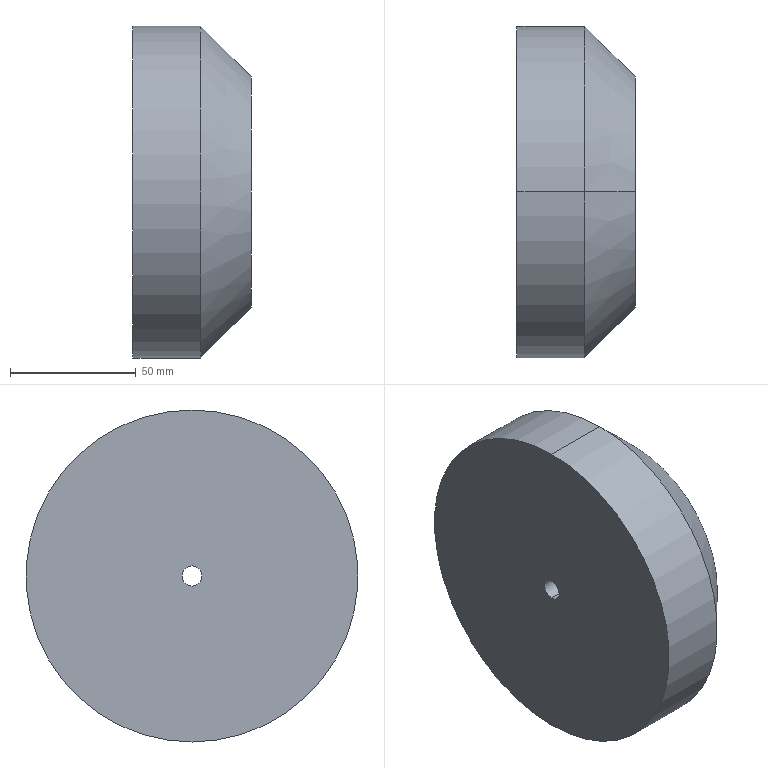Part | STEP file | PRODUCT_NAME_45_default | 1 solid | 8 faces | box 47 x 132 x 132 mm | volume 566262 mm3 | cylinder 4 | cone 2 | plane 2 | commonest cylinder face diameters 8 x2 132 x2
STEP:
#1=CARTESIAN_POINT('',(0.,0.,0.));
#2=DIRECTION('',(0.,0.,1.));
#3=DIRECTION('',(1.,0.,0.));
#4=AXIS2_PLACEMENT_3D('',#1,#2,#3);
#5=CARTESIAN_POINT('',(224.,57.,66.));
#6=VERTEX_POINT('',#5);
#7=CARTESIAN_POINT('',(224.,57.,-66.));
#8=VERTEX_POINT('',#7);
#9=CARTESIAN_POINT('',(224.,57.,0.));
#10=DIRECTION('',(-1.,0.,0.));
#11=DIRECTION('',(0.,0.,-1.));
#12=AXIS2_PLACEMENT_3D('',#9,#10,#11);
#13=CIRCLE('',#12,66.);
#14=CARTESIAN_POINT('',(237.5,57.,0.));
#15=DIRECTION('',(1.,0.,0.));
#16=DIRECTION('',(0.,0.,-1.));
#17=AXIS2_PLACEMENT_3D('',#14,#15,#16);
#18=CYLINDRICAL_SURFACE('',#17,66.);
#19=CARTESIAN_POINT('',(6.283,-13.5));
#20=DIRECTION('',(-1.,0.));
#21=VECTOR('',#20,1.);
#22=LINE('',#19,#21);
#23=(GEOMETRIC_REPRESENTATION_CONTEXT(2)PARAMETRIC_REPRESENTATION_CONTEXT()REPRESENTATION_CONTEXT('',''));
#24=DEFINITIONAL_REPRESENTATION('',(#22),#23);
#25=PCURVE('',#18,#24);
#26=CARTESIAN_POINT('',(224.,57.,0.));
#27=DIRECTION('',(-1.,0.,0.));
#28=DIRECTION('',(0.,0.,1.));
#29=AXIS2_PLACEMENT_3D('',#26,#27,#28);
#30=PLANE('',#29);
#31=CARTESIAN_POINT('',(0.,0.));
#32=DIRECTION('',(-1.,0.));
#33=AXIS2_PLACEMENT_2D('',#31,#32);
#34=CIRCLE('',#33,66.);
#35=(GEOMETRIC_REPRESENTATION_CONTEXT(2)PARAMETRIC_REPRESENTATION_CONTEXT()REPRESENTATION_CONTEXT('',''));
#36=DEFINITIONAL_REPRESENTATION('',(#34),#35);
#37=PCURVE('',#30,#36);
#38=SURFACE_CURVE('',#13,(#25,#37),.PCURVE_S1.);
#39=EDGE_CURVE('',#6,#8,#38,.T.);
#40=ORIENTED_EDGE('',*,*,#39,.F.);
#41=CARTESIAN_POINT('',(251.,57.,66.));
#42=VERTEX_POINT('',#41);
#43=CARTESIAN_POINT('',(237.5,57.,66.));
#44=DIRECTION('',(1.,0.,0.));
#45=VECTOR('',#44,1.);
#46=LINE('',#43,#45);
#47=CARTESIAN_POINT('',(3.142,0.));
#48=DIRECTION('',(0.,1.));
#49=VECTOR('',#48,1.);
#50=LINE('',#47,#49);
#51=(GEOMETRIC_REPRESENTATION_CONTEXT(2)PARAMETRIC_REPRESENTATION_CONTEXT()REPRESENTATION_CONTEXT('',''));
#52=DEFINITIONAL_REPRESENTATION('',(#50),#51);
#53=PCURVE('',#18,#52);
#54=CARTESIAN_POINT('',(237.5,57.,0.));
#55=DIRECTION('',(1.,0.,0.));
#56=DIRECTION('',(0.,0.,-1.));
#57=AXIS2_PLACEMENT_3D('',#54,#55,#56);
#58=CYLINDRICAL_SURFACE('',#57,66.);
#59=CARTESIAN_POINT('',(3.142,0.));
#60=DIRECTION('',(0.,1.));
#61=VECTOR('',#60,1.);
#62=LINE('',#59,#61);
#63=(GEOMETRIC_REPRESENTATION_CONTEXT(2)PARAMETRIC_REPRESENTATION_CONTEXT()REPRESENTATION_CONTEXT('',''));
#64=DEFINITIONAL_REPRESENTATION('',(#62),#63);
#65=PCURVE('',#58,#64);
#66=SURFACE_CURVE('',#46,(#53,#65),.PCURVE_S1.);
#67=EDGE_CURVE('',#6,#42,#66,.T.);
#68=ORIENTED_EDGE('',*,*,#67,.T.);
#69=CARTESIAN_POINT('',(251.,57.,-66.));
#70=VERTEX_POINT('',#69);
#71=CARTESIAN_POINT('',(251.,57.,0.));
#72=DIRECTION('',(-1.,0.,0.));
#73=DIRECTION('',(0.,0.,-1.));
#74=AXIS2_PLACEMENT_3D('',#71,#72,#73);
#75=CIRCLE('',#74,66.);
#76=CARTESIAN_POINT('',(6.283,13.5));
#77=DIRECTION('',(-1.,0.));
#78=VECTOR('',#77,1.);
#79=LINE('',#76,#78);
#80=(GEOMETRIC_REPRESENTATION_CONTEXT(2)PARAMETRIC_REPRESENTATION_CONTEXT()REPRESENTATION_CONTEXT('',''));
#81=DEFINITIONAL_REPRESENTATION('',(#79),#80);
#82=PCURVE('',#18,#81);
#83=CARTESIAN_POINT('',(251.,57.,0.));
#84=DIRECTION('',(-1.,0.,0.));
#85=DIRECTION('',(0.,0.,1.));
#86=AXIS2_PLACEMENT_3D('',#83,#84,#85);
#87=CONICAL_SURFACE('',#86,66.,0.7854);
#88=CARTESIAN_POINT('',(-3.142,0.));
#89=DIRECTION('',(1.,0.));
#90=VECTOR('',#89,1.);
#91=LINE('',#88,#90);
#92=(GEOMETRIC_REPRESENTATION_CONTEXT(2)PARAMETRIC_REPRESENTATION_CONTEXT()REPRESENTATION_CONTEXT('',''));
#93=DEFINITIONAL_REPRESENTATION('',(#91),#92);
#94=PCURVE('',#87,#93);
#95=SURFACE_CURVE('',#75,(#82,#94),.PCURVE_S1.);
#96=EDGE_CURVE('',#42,#70,#95,.T.);
#97=ORIENTED_EDGE('',*,*,#96,.T.);
#98=CARTESIAN_POINT('',(237.5,57.,-66.));
#99=DIRECTION('',(1.,0.,0.));
#100=VECTOR('',#99,1.);
#101=LINE('',#98,#100);
#102=CARTESIAN_POINT('',(0.,0.));
#103=DIRECTION('',(0.,1.));
#104=VECTOR('',#103,1.);
#105=LINE('',#102,#104);
#106=(GEOMETRIC_REPRESENTATION_CONTEXT(2)PARAMETRIC_REPRESENTATION_CONTEXT()REPRESENTATION_CONTEXT('',''));
#107=DEFINITIONAL_REPRESENTATION('',(#105),#106);
#108=PCURVE('',#18,#107);
#109=CARTESIAN_POINT('',(6.283,0.));
#110=DIRECTION('',(0.,1.));
#111=VECTOR('',#110,1.);
#112=LINE('',#109,#111);
#113=(GEOMETRIC_REPRESENTATION_CONTEXT(2)PARAMETRIC_REPRESENTATION_CONTEXT()REPRESENTATION_CONTEXT('',''));
#114=DEFINITIONAL_REPRESENTATION('',(#112),#113);
#115=PCURVE('',#58,#114);
#116=SURFACE_CURVE('',#101,(#108,#115),.PCURVE_S1.);
#117=EDGE_CURVE('',#8,#70,#116,.T.);
#118=ORIENTED_EDGE('',*,*,#117,.F.);
#119=EDGE_LOOP('',(#40,#68,#97,#118));
#120=FACE_BOUND('',#119,.T.);
#121=ADVANCED_FACE('',(#120),#18,.T.);
#122=CARTESIAN_POINT('',(224.,57.,-4.));
#123=VERTEX_POINT('',#122);
#124=CARTESIAN_POINT('',(271.,57.,-4.));
#125=VERTEX_POINT('',#124);
#126=CARTESIAN_POINT('',(247.5,57.,-4.));
#127=DIRECTION('',(1.,0.,0.));
#128=VECTOR('',#127,1.);
#129=LINE('',#126,#128);
#130=CARTESIAN_POINT('',(247.5,57.,0.));
#131=DIRECTION('',(1.,0.,0.));
#132=DIRECTION('',(0.,0.,-1.));
#133=AXIS2_PLACEMENT_3D('',#130,#131,#132);
#134=CYLINDRICAL_SURFACE('',#133,4.);
#135=CARTESIAN_POINT('',(6.283,0.));
#136=DIRECTION('',(0.,1.));
#137=VECTOR('',#136,1.);
#138=LINE('',#135,#137);
#139=(GEOMETRIC_REPRESENTATION_CONTEXT(2)PARAMETRIC_REPRESENTATION_CONTEXT()REPRESENTATION_CONTEXT('',''));
#140=DEFINITIONAL_REPRESENTATION('',(#138),#139);
#141=PCURVE('',#134,#140);
#142=CARTESIAN_POINT('',(247.5,57.,0.));
#143=DIRECTION('',(1.,0.,0.));
#144=DIRECTION('',(0.,0.,-1.));
#145=AXIS2_PLACEMENT_3D('',#142,#143,#144);
#146=CYLINDRICAL_SURFACE('',#145,4.);
#147=CARTESIAN_POINT('',(0.,0.));
#148=DIRECTION('',(0.,1.));
#149=VECTOR('',#148,1.);
#150=LINE('',#147,#149);
#151=(GEOMETRIC_REPRESENTATION_CONTEXT(2)PARAMETRIC_REPRESENTATION_CONTEXT()REPRESENTATION_CONTEXT('',''));
#152=DEFINITIONAL_REPRESENTATION('',(#150),#151);
#153=PCURVE('',#146,#152);
#154=SURFACE_CURVE('',#129,(#141,#153),.PCURVE_S1.);
#155=EDGE_CURVE('',#123,#125,#154,.T.);
#156=ORIENTED_EDGE('',*,*,#155,.T.);
#157=CARTESIAN_POINT('',(271.,57.,4.));
#158=VERTEX_POINT('',#157);
#159=CARTESIAN_POINT('',(271.,57.,0.));
#160=DIRECTION('',(-1.,0.,0.));
#161=DIRECTION('',(0.,0.,-1.));
#162=AXIS2_PLACEMENT_3D('',#159,#160,#161);
#163=CIRCLE('',#162,4.);
#164=CARTESIAN_POINT('',(6.283,23.5));
#165=DIRECTION('',(-1.,0.));
#166=VECTOR('',#165,1.);
#167=LINE('',#164,#166);
#168=(GEOMETRIC_REPRESENTATION_CONTEXT(2)PARAMETRIC_REPRESENTATION_CONTEXT()REPRESENTATION_CONTEXT('',''));
#169=DEFINITIONAL_REPRESENTATION('',(#167),#168);
#170=PCURVE('',#134,#169);
#171=CARTESIAN_POINT('',(271.,57.,0.));
#172=DIRECTION('',(-1.,0.,0.));
#173=DIRECTION('',(0.,0.,1.));
#174=AXIS2_PLACEMENT_3D('',#171,#172,#173);
#175=PLANE('',#174);
#176=CARTESIAN_POINT('',(0.,0.));
#177=DIRECTION('',(-1.,0.));
#178=AXIS2_PLACEMENT_2D('',#176,#177);
#179=CIRCLE('',#178,4.);
#180=(GEOMETRIC_REPRESENTATION_CONTEXT(2)PARAMETRIC_REPRESENTATION_CONTEXT()REPRESENTATION_CONTEXT('',''));
#181=DEFINITIONAL_REPRESENTATION('',(#179),#180);
#182=PCURVE('',#175,#181);
#183=SURFACE_CURVE('',#163,(#170,#182),.PCURVE_S1.);
#184=EDGE_CURVE('',#125,#158,#183,.T.);
#185=ORIENTED_EDGE('',*,*,#184,.T.);
#186=CARTESIAN_POINT('',(224.,57.,4.));
#187=VERTEX_POINT('',#186);
#188=CARTESIAN_POINT('',(247.5,57.,4.));
#189=DIRECTION('',(1.,0.,0.));
#190=VECTOR('',#189,1.);
#191=LINE('',#188,#190);
#192=CARTESIAN_POINT('',(3.142,0.));
#193=DIRECTION('',(0.,1.));
#194=VECTOR('',#193,1.);
#195=LINE('',#192,#194);
#196=(GEOMETRIC_REPRESENTATION_CONTEXT(2)PARAMETRIC_REPRESENTATION_CONTEXT()REPRESENTATION_CONTEXT('',''));
#197=DEFINITIONAL_REPRESENTATION('',(#195),#196);
#198=PCURVE('',#134,#197);
#199=CARTESIAN_POINT('',(3.142,0.));
#200=DIRECTION('',(0.,1.));
#201=VECTOR('',#200,1.);
#202=LINE('',#199,#201);
#203=(GEOMETRIC_REPRESENTATION_CONTEXT(2)PARAMETRIC_REPRESENTATION_CONTEXT()REPRESENTATION_CONTEXT('',''));
#204=DEFINITIONAL_REPRESENTATION('',(#202),#203);
#205=PCURVE('',#146,#204);
#206=SURFACE_CURVE('',#191,(#198,#205),.PCURVE_S1.);
#207=EDGE_CURVE('',#187,#158,#206,.T.);
#208=ORIENTED_EDGE('',*,*,#207,.F.);
#209=CARTESIAN_POINT('',(224.,57.,0.));
#210=DIRECTION('',(1.,0.,0.));
#211=DIRECTION('',(0.,0.,-1.));
#212=AXIS2_PLACEMENT_3D('',#209,#210,#211);
#213=CIRCLE('',#212,4.);
#214=CARTESIAN_POINT('',(0.,-23.5));
#215=DIRECTION('',(1.,0.));
#216=VECTOR('',#215,1.);
#217=LINE('',#214,#216);
#218=(GEOMETRIC_REPRESENTATION_CONTEXT(2)PARAMETRIC_REPRESENTATION_CONTEXT()REPRESENTATION_CONTEXT('',''));
#219=DEFINITIONAL_REPRESENTATION('',(#217),#218);
#220=PCURVE('',#134,#219);
#221=CARTESIAN_POINT('',(-4.,0.));
#222=CARTESIAN_POINT('',(-4.,6.928));
#223=CARTESIAN_POINT('',(2.,3.464));
#224=CARTESIAN_POINT('',(8.,0.));
#225=CARTESIAN_POINT('',(2.,-3.464));
#226=CARTESIAN_POINT('',(-4.,-6.928));
#227=CARTESIAN_POINT('',(-4.,0.));
#228=(BOUNDED_CURVE()B_SPLINE_CURVE(2,(#221,#222,#223,#224,#225,#226,#227),.UNSPECIFIED.,.T.,.F.)B_SPLINE_CURVE_WITH_KNOTS((1,2,2,2,2,1),(-2.094,0.,2.094,4.189,6.283,8.378),.UNSPECIFIED.)CURVE()GEOMETRIC_REPRESENTATION_ITEM()RATIONAL_B_SPLINE_CURVE((1.,0.5,1.,0.5,1.,0.5,1.))REPRESENTATION_ITEM(''));
#229=(GEOMETRIC_REPRESENTATION_CONTEXT(2)PARAMETRIC_REPRESENTATION_CONTEXT()REPRESENTATION_CONTEXT('',''));
#230=DEFINITIONAL_REPRESENTATION('',(#228),#229);
#231=PCURVE('',#30,#230);
#232=SURFACE_CURVE('',#213,(#220,#231),.PCURVE_S1.);
#233=EDGE_CURVE('',#187,#123,#232,.T.);
#234=ORIENTED_EDGE('',*,*,#233,.T.);
#235=EDGE_LOOP('',(#156,#185,#208,#234));
#236=FACE_BOUND('',#235,.F.);
#237=ADVANCED_FACE('',(#236),#134,.F.);
#238=CARTESIAN_POINT('',(271.,57.,46.));
#239=VERTEX_POINT('',#238);
#240=CARTESIAN_POINT('',(271.,57.,-46.));
#241=VERTEX_POINT('',#240);
#242=CARTESIAN_POINT('',(271.,57.,0.));
#243=DIRECTION('',(-1.,0.,0.));
#244=DIRECTION('',(0.,0.,1.));
#245=AXIS2_PLACEMENT_3D('',#242,#243,#244);
#246=CIRCLE('',#245,46.);
#247=CARTESIAN_POINT('',(0.,-20.));
#248=DIRECTION('',(1.,0.));
#249=VECTOR('',#248,1.);
#250=LINE('',#247,#249);
#251=(GEOMETRIC_REPRESENTATION_CONTEXT(2)PARAMETRIC_REPRESENTATION_CONTEXT()REPRESENTATION_CONTEXT('',''));
#252=DEFINITIONAL_REPRESENTATION('',(#250),#251);
#253=PCURVE('',#87,#252);
#254=CARTESIAN_POINT('',(0.,0.));
#255=DIRECTION('',(1.,0.));
#256=AXIS2_PLACEMENT_2D('',#254,#255);
#257=CIRCLE('',#256,46.);
#258=(GEOMETRIC_REPRESENTATION_CONTEXT(2)PARAMETRIC_REPRESENTATION_CONTEXT()REPRESENTATION_CONTEXT('',''));
#259=DEFINITIONAL_REPRESENTATION('',(#257),#258);
#260=PCURVE('',#175,#259);
#261=SURFACE_CURVE('',#246,(#253,#260),.PCURVE_S1.);
#262=EDGE_CURVE('',#239,#241,#261,.T.);
#263=ORIENTED_EDGE('',*,*,#262,.T.);
#264=CARTESIAN_POINT('',(251.,57.,-66.));
#265=DIRECTION('',(-0.7071,0.,-0.7071));
#266=VECTOR('',#265,1.);
#267=LINE('',#264,#266);
#268=CARTESIAN_POINT('',(3.142,0.));
#269=DIRECTION('',(0.,1.));
#270=VECTOR('',#269,1.);
#271=LINE('',#268,#270);
#272=(GEOMETRIC_REPRESENTATION_CONTEXT(2)PARAMETRIC_REPRESENTATION_CONTEXT()REPRESENTATION_CONTEXT('',''));
#273=DEFINITIONAL_REPRESENTATION('',(#271),#272);
#274=PCURVE('',#87,#273);
#275=CARTESIAN_POINT('',(251.,57.,0.));
#276=DIRECTION('',(-1.,0.,0.));
#277=DIRECTION('',(0.,0.,1.));
#278=AXIS2_PLACEMENT_3D('',#275,#276,#277);
#279=CONICAL_SURFACE('',#278,66.,0.7854);
#280=CARTESIAN_POINT('',(3.142,0.));
#281=DIRECTION('',(0.,1.));
#282=VECTOR('',#281,1.);
#283=LINE('',#280,#282);
#284=(GEOMETRIC_REPRESENTATION_CONTEXT(2)PARAMETRIC_REPRESENTATION_CONTEXT()REPRESENTATION_CONTEXT('',''));
#285=DEFINITIONAL_REPRESENTATION('',(#283),#284);
#286=PCURVE('',#279,#285);
#287=SURFACE_CURVE('',#267,(#274,#286),.PCURVE_S1.);
#288=EDGE_CURVE('',#241,#70,#287,.T.);
#289=ORIENTED_EDGE('',*,*,#288,.T.);
#290=ORIENTED_EDGE('',*,*,#96,.F.);
#291=CARTESIAN_POINT('',(251.,57.,66.));
#292=DIRECTION('',(-0.7071,0.,0.7071));
#293=VECTOR('',#292,1.);
#294=LINE('',#291,#293);
#295=CARTESIAN_POINT('',(0.,0.));
#296=DIRECTION('',(0.,1.));
#297=VECTOR('',#296,1.);
#298=LINE('',#295,#297);
#299=(GEOMETRIC_REPRESENTATION_CONTEXT(2)PARAMETRIC_REPRESENTATION_CONTEXT()REPRESENTATION_CONTEXT('',''));
#300=DEFINITIONAL_REPRESENTATION('',(#298),#299);
#301=PCURVE('',#87,#300);
#302=CARTESIAN_POINT('',(6.283,0.));
#303=DIRECTION('',(0.,1.));
#304=VECTOR('',#303,1.);
#305=LINE('',#302,#304);
#306=(GEOMETRIC_REPRESENTATION_CONTEXT(2)PARAMETRIC_REPRESENTATION_CONTEXT()REPRESENTATION_CONTEXT('',''));
#307=DEFINITIONAL_REPRESENTATION('',(#305),#306);
#308=PCURVE('',#279,#307);
#309=SURFACE_CURVE('',#294,(#301,#308),.PCURVE_S1.);
#310=EDGE_CURVE('',#239,#42,#309,.T.);
#311=ORIENTED_EDGE('',*,*,#310,.F.);
#312=EDGE_LOOP('',(#263,#289,#290,#311));
#313=FACE_BOUND('',#312,.T.);
#314=ADVANCED_FACE('',(#313),#87,.T.);
#315=CARTESIAN_POINT('',(224.,57.,0.));
#316=DIRECTION('',(-1.,0.,0.));
#317=DIRECTION('',(0.,0.,-1.));
#318=AXIS2_PLACEMENT_3D('',#315,#316,#317);
#319=CIRCLE('',#318,66.);
#320=CARTESIAN_POINT('',(0.,0.));
#321=DIRECTION('',(-1.,0.));
#322=AXIS2_PLACEMENT_2D('',#320,#321);
#323=CIRCLE('',#322,66.);
#324=(GEOMETRIC_REPRESENTATION_CONTEXT(2)PARAMETRIC_REPRESENTATION_CONTEXT()REPRESENTATION_CONTEXT('',''));
#325=DEFINITIONAL_REPRESENTATION('',(#323),#324);
#326=PCURVE('',#30,#325);
#327=CARTESIAN_POINT('',(6.283,-13.5));
#328=DIRECTION('',(-1.,0.));
#329=VECTOR('',#328,1.);
#330=LINE('',#327,#329);
#331=(GEOMETRIC_REPRESENTATION_CONTEXT(2)PARAMETRIC_REPRESENTATION_CONTEXT()REPRESENTATION_CONTEXT('',''));
#332=DEFINITIONAL_REPRESENTATION('',(#330),#331);
#333=PCURVE('',#58,#332);
#334=SURFACE_CURVE('',#319,(#326,#333),.PCURVE_S1.);
#335=EDGE_CURVE('',#8,#6,#334,.T.);
#336=ORIENTED_EDGE('',*,*,#335,.T.);
#337=ORIENTED_EDGE('',*,*,#39,.T.);
#338=EDGE_LOOP('',(#336,#337));
#339=FACE_BOUND('',#338,.T.);
#340=CARTESIAN_POINT('',(224.,57.,0.));
#341=DIRECTION('',(1.,0.,0.));
#342=DIRECTION('',(0.,0.,-1.));
#343=AXIS2_PLACEMENT_3D('',#340,#341,#342);
#344=CIRCLE('',#343,4.);
#345=CARTESIAN_POINT('',(-4.,0.));
#346=CARTESIAN_POINT('',(-4.,6.928));
#347=CARTESIAN_POINT('',(2.,3.464));
#348=CARTESIAN_POINT('',(8.,0.));
#349=CARTESIAN_POINT('',(2.,-3.464));
#350=CARTESIAN_POINT('',(-4.,-6.928));
#351=CARTESIAN_POINT('',(-4.,0.));
#352=(BOUNDED_CURVE()B_SPLINE_CURVE(2,(#345,#346,#347,#348,#349,#350,#351),.UNSPECIFIED.,.T.,.F.)B_SPLINE_CURVE_WITH_KNOTS((1,2,2,2,2,1),(-2.094,0.,2.094,4.189,6.283,8.378),.UNSPECIFIED.)CURVE()GEOMETRIC_REPRESENTATION_ITEM()RATIONAL_B_SPLINE_CURVE((1.,0.5,1.,0.5,1.,0.5,1.))REPRESENTATION_ITEM(''));
#353=(GEOMETRIC_REPRESENTATION_CONTEXT(2)PARAMETRIC_REPRESENTATION_CONTEXT()REPRESENTATION_CONTEXT('',''));
#354=DEFINITIONAL_REPRESENTATION('',(#352),#353);
#355=PCURVE('',#30,#354);
#356=CARTESIAN_POINT('',(0.,-23.5));
#357=DIRECTION('',(1.,0.));
#358=VECTOR('',#357,1.);
#359=LINE('',#356,#358);
#360=(GEOMETRIC_REPRESENTATION_CONTEXT(2)PARAMETRIC_REPRESENTATION_CONTEXT()REPRESENTATION_CONTEXT('',''));
#361=DEFINITIONAL_REPRESENTATION('',(#359),#360);
#362=PCURVE('',#146,#361);
#363=SURFACE_CURVE('',#344,(#355,#362),.PCURVE_S1.);
#364=EDGE_CURVE('',#123,#187,#363,.T.);
#365=ORIENTED_EDGE('',*,*,#364,.T.);
#366=ORIENTED_EDGE('',*,*,#233,.T.);
#367=EDGE_LOOP('',(#365,#366));
#368=FACE_BOUND('',#367,.T.);
#369=ADVANCED_FACE('',(#339,#368),#30,.T.);
#370=ORIENTED_EDGE('',*,*,#67,.F.);
#371=ORIENTED_EDGE('',*,*,#335,.F.);
#372=ORIENTED_EDGE('',*,*,#117,.T.);
#373=CARTESIAN_POINT('',(251.,57.,0.));
#374=DIRECTION('',(-1.,0.,0.));
#375=DIRECTION('',(0.,0.,-1.));
#376=AXIS2_PLACEMENT_3D('',#373,#374,#375);
#377=CIRCLE('',#376,66.);
#378=CARTESIAN_POINT('',(6.283,13.5));
#379=DIRECTION('',(-1.,0.));
#380=VECTOR('',#379,1.);
#381=LINE('',#378,#380);
#382=(GEOMETRIC_REPRESENTATION_CONTEXT(2)PARAMETRIC_REPRESENTATION_CONTEXT()REPRESENTATION_CONTEXT('',''));
#383=DEFINITIONAL_REPRESENTATION('',(#381),#382);
#384=PCURVE('',#58,#383);
#385=CARTESIAN_POINT('',(3.142,0.));
#386=DIRECTION('',(1.,0.));
#387=VECTOR('',#386,1.);
#388=LINE('',#385,#387);
#389=(GEOMETRIC_REPRESENTATION_CONTEXT(2)PARAMETRIC_REPRESENTATION_CONTEXT()REPRESENTATION_CONTEXT('',''));
#390=DEFINITIONAL_REPRESENTATION('',(#388),#389);
#391=PCURVE('',#279,#390);
#392=SURFACE_CURVE('',#377,(#384,#391),.PCURVE_S1.);
#393=EDGE_CURVE('',#70,#42,#392,.T.);
#394=ORIENTED_EDGE('',*,*,#393,.T.);
#395=EDGE_LOOP('',(#370,#371,#372,#394));
#396=FACE_BOUND('',#395,.T.);
#397=ADVANCED_FACE('',(#396),#58,.T.);
#398=CARTESIAN_POINT('',(271.,57.,0.));
#399=DIRECTION('',(-1.,0.,0.));
#400=DIRECTION('',(0.,0.,-1.));
#401=AXIS2_PLACEMENT_3D('',#398,#399,#400);
#402=CIRCLE('',#401,4.);
#403=CARTESIAN_POINT('',(6.283,23.5));
#404=DIRECTION('',(-1.,0.));
#405=VECTOR('',#404,1.);
#406=LINE('',#403,#405);
#407=(GEOMETRIC_REPRESENTATION_CONTEXT(2)PARAMETRIC_REPRESENTATION_CONTEXT()REPRESENTATION_CONTEXT('',''));
#408=DEFINITIONAL_REPRESENTATION('',(#406),#407);
#409=PCURVE('',#146,#408);
#410=CARTESIAN_POINT('',(0.,0.));
#411=DIRECTION('',(-1.,0.));
#412=AXIS2_PLACEMENT_2D('',#410,#411);
#413=CIRCLE('',#412,4.);
#414=(GEOMETRIC_REPRESENTATION_CONTEXT(2)PARAMETRIC_REPRESENTATION_CONTEXT()REPRESENTATION_CONTEXT('',''));
#415=DEFINITIONAL_REPRESENTATION('',(#413),#414);
#416=PCURVE('',#175,#415);
#417=SURFACE_CURVE('',#402,(#409,#416),.PCURVE_S1.);
#418=EDGE_CURVE('',#158,#125,#417,.T.);
#419=ORIENTED_EDGE('',*,*,#418,.T.);
#420=ORIENTED_EDGE('',*,*,#155,.F.);
#421=ORIENTED_EDGE('',*,*,#364,.T.);
#422=ORIENTED_EDGE('',*,*,#207,.T.);
#423=EDGE_LOOP('',(#419,#420,#421,#422));
#424=FACE_BOUND('',#423,.F.);
#425=ADVANCED_FACE('',(#424),#146,.F.);
#426=ORIENTED_EDGE('',*,*,#288,.F.);
#427=CARTESIAN_POINT('',(271.,57.,0.));
#428=DIRECTION('',(-1.,0.,0.));
#429=DIRECTION('',(0.,0.,1.));
#430=AXIS2_PLACEMENT_3D('',#427,#428,#429);
#431=CIRCLE('',#430,46.);
#432=CARTESIAN_POINT('',(0.,-20.));
#433=DIRECTION('',(1.,0.));
#434=VECTOR('',#433,1.);
#435=LINE('',#432,#434);
#436=(GEOMETRIC_REPRESENTATION_CONTEXT(2)PARAMETRIC_REPRESENTATION_CONTEXT()REPRESENTATION_CONTEXT('',''));
#437=DEFINITIONAL_REPRESENTATION('',(#435),#436);
#438=PCURVE('',#279,#437);
#439=CARTESIAN_POINT('',(0.,0.));
#440=DIRECTION('',(1.,0.));
#441=AXIS2_PLACEMENT_2D('',#439,#440);
#442=CIRCLE('',#441,46.);
#443=(GEOMETRIC_REPRESENTATION_CONTEXT(2)PARAMETRIC_REPRESENTATION_CONTEXT()REPRESENTATION_CONTEXT('',''));
#444=DEFINITIONAL_REPRESENTATION('',(#442),#443);
#445=PCURVE('',#175,#444);
#446=SURFACE_CURVE('',#431,(#438,#445),.PCURVE_S1.);
#447=EDGE_CURVE('',#241,#239,#446,.T.);
#448=ORIENTED_EDGE('',*,*,#447,.T.);
#449=ORIENTED_EDGE('',*,*,#310,.T.);
#450=ORIENTED_EDGE('',*,*,#393,.F.);
#451=EDGE_LOOP('',(#426,#448,#449,#450));
#452=FACE_BOUND('',#451,.T.);
#453=ADVANCED_FACE('',(#452),#279,.T.);
#454=ORIENTED_EDGE('',*,*,#262,.F.);
#455=ORIENTED_EDGE('',*,*,#447,.F.);
#456=EDGE_LOOP('',(#454,#455));
#457=FACE_BOUND('',#456,.T.);
#458=ORIENTED_EDGE('',*,*,#184,.T.);
#459=ORIENTED_EDGE('',*,*,#418,.T.);
#460=EDGE_LOOP('',(#458,#459));
#461=FACE_BOUND('',#460,.T.);
#462=ADVANCED_FACE('',(#457,#461),#175,.F.);
#463=CLOSED_SHELL('',(#121,#237,#314,#369,#397,#425,#453,#462));
#464=MANIFOLD_SOLID_BREP('',#463);
#465=(LENGTH_UNIT()NAMED_UNIT(*)SI_UNIT(.MILLI.,.METRE.));
#466=UNCERTAINTY_MEASURE_WITH_UNIT(LENGTH_MEASURE(0.0000001),#465,'','');
#467=(NAMED_UNIT(*)PLANE_ANGLE_UNIT()SI_UNIT($,.RADIAN.));
#468=(NAMED_UNIT(*)SI_UNIT($,.STERADIAN.)SOLID_ANGLE_UNIT());
#469=(GEOMETRIC_REPRESENTATION_CONTEXT(3)GLOBAL_UNCERTAINTY_ASSIGNED_CONTEXT((#466))GLOBAL_UNIT_ASSIGNED_CONTEXT((#465,#467,#468))REPRESENTATION_CONTEXT('',''));
#470=ADVANCED_BREP_SHAPE_REPRESENTATION('',(#4,#464),#469);